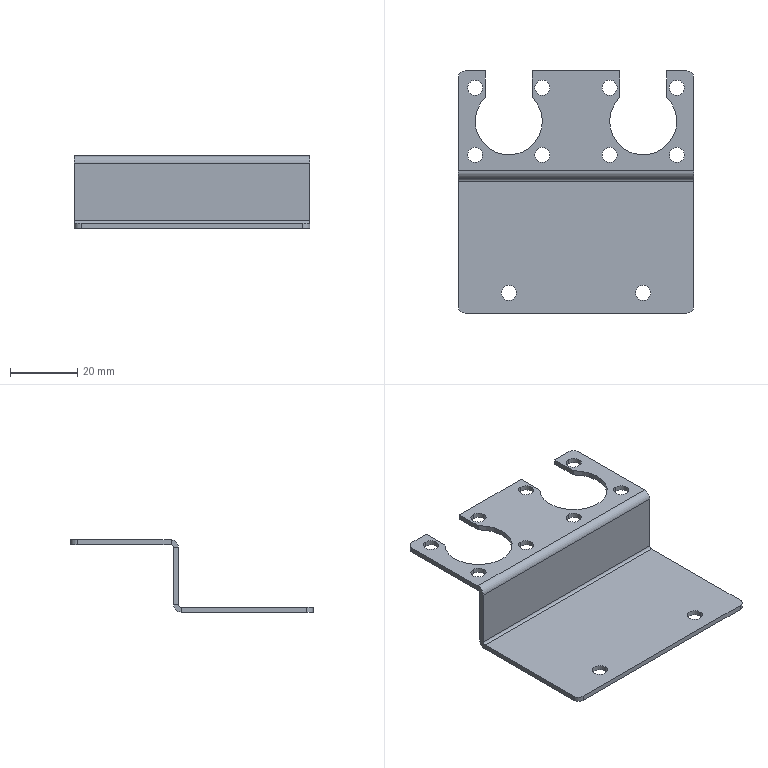Part | STEP file | 02-21 vacuum gauge mounting seat (Default) | 1 solid | 54 faces | box 70 x 72 x 21.5 mm | volume 8092 mm3 | cylinder 30 | plane 24 | commonest cylinder face diameters 4.5 x20 4 x4 1.473 x2 4.473 x2 20 x2